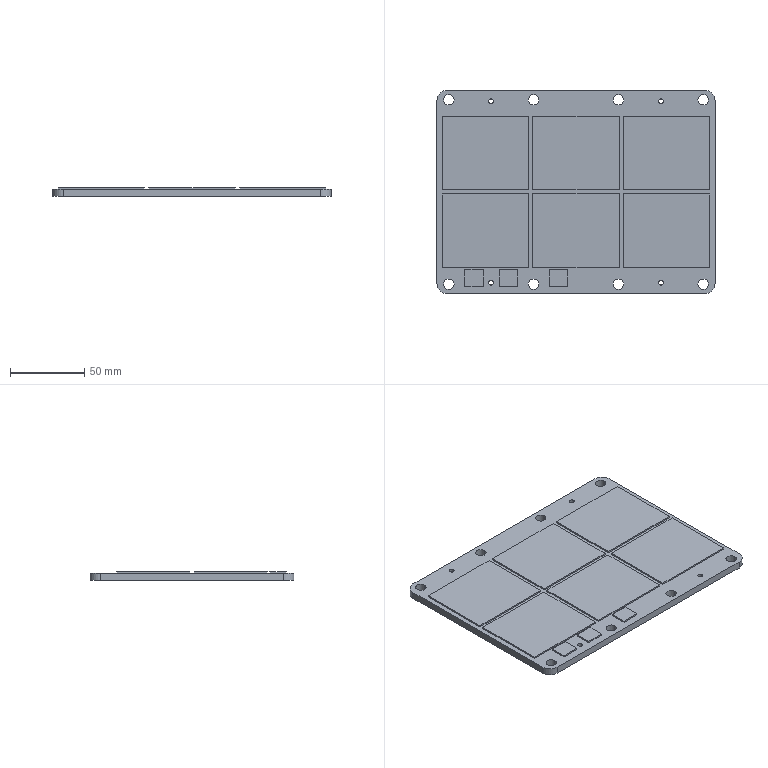Part | SolidWorks | features ICE 3, HoleWzd 2, Extrusion 1, Fillet 1 | 1 solid | 79 faces | box 187 x 137 x 5.87 mm | volume 140466 mm3 | plane 51 | cylinder 28 | commonest cylinder face diameters 7 x16 3.2 x8 14 x4